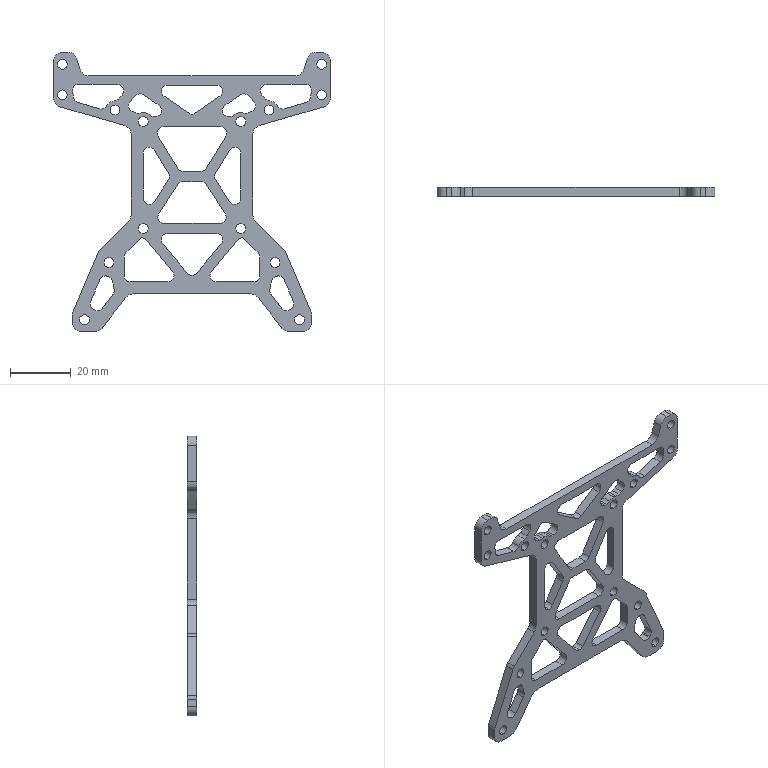Part | SolidWorks | features Fillet 2, Extrusion 1, ICE 1 | 1 solid | 201 faces | box 91 x 3 x 91.75 mm | volume 7865 mm3 | cylinder 129 | plane 72 | commonest cylinder face diameters 4 x67 3.2 x28 6 x28 9 x4 7 x2